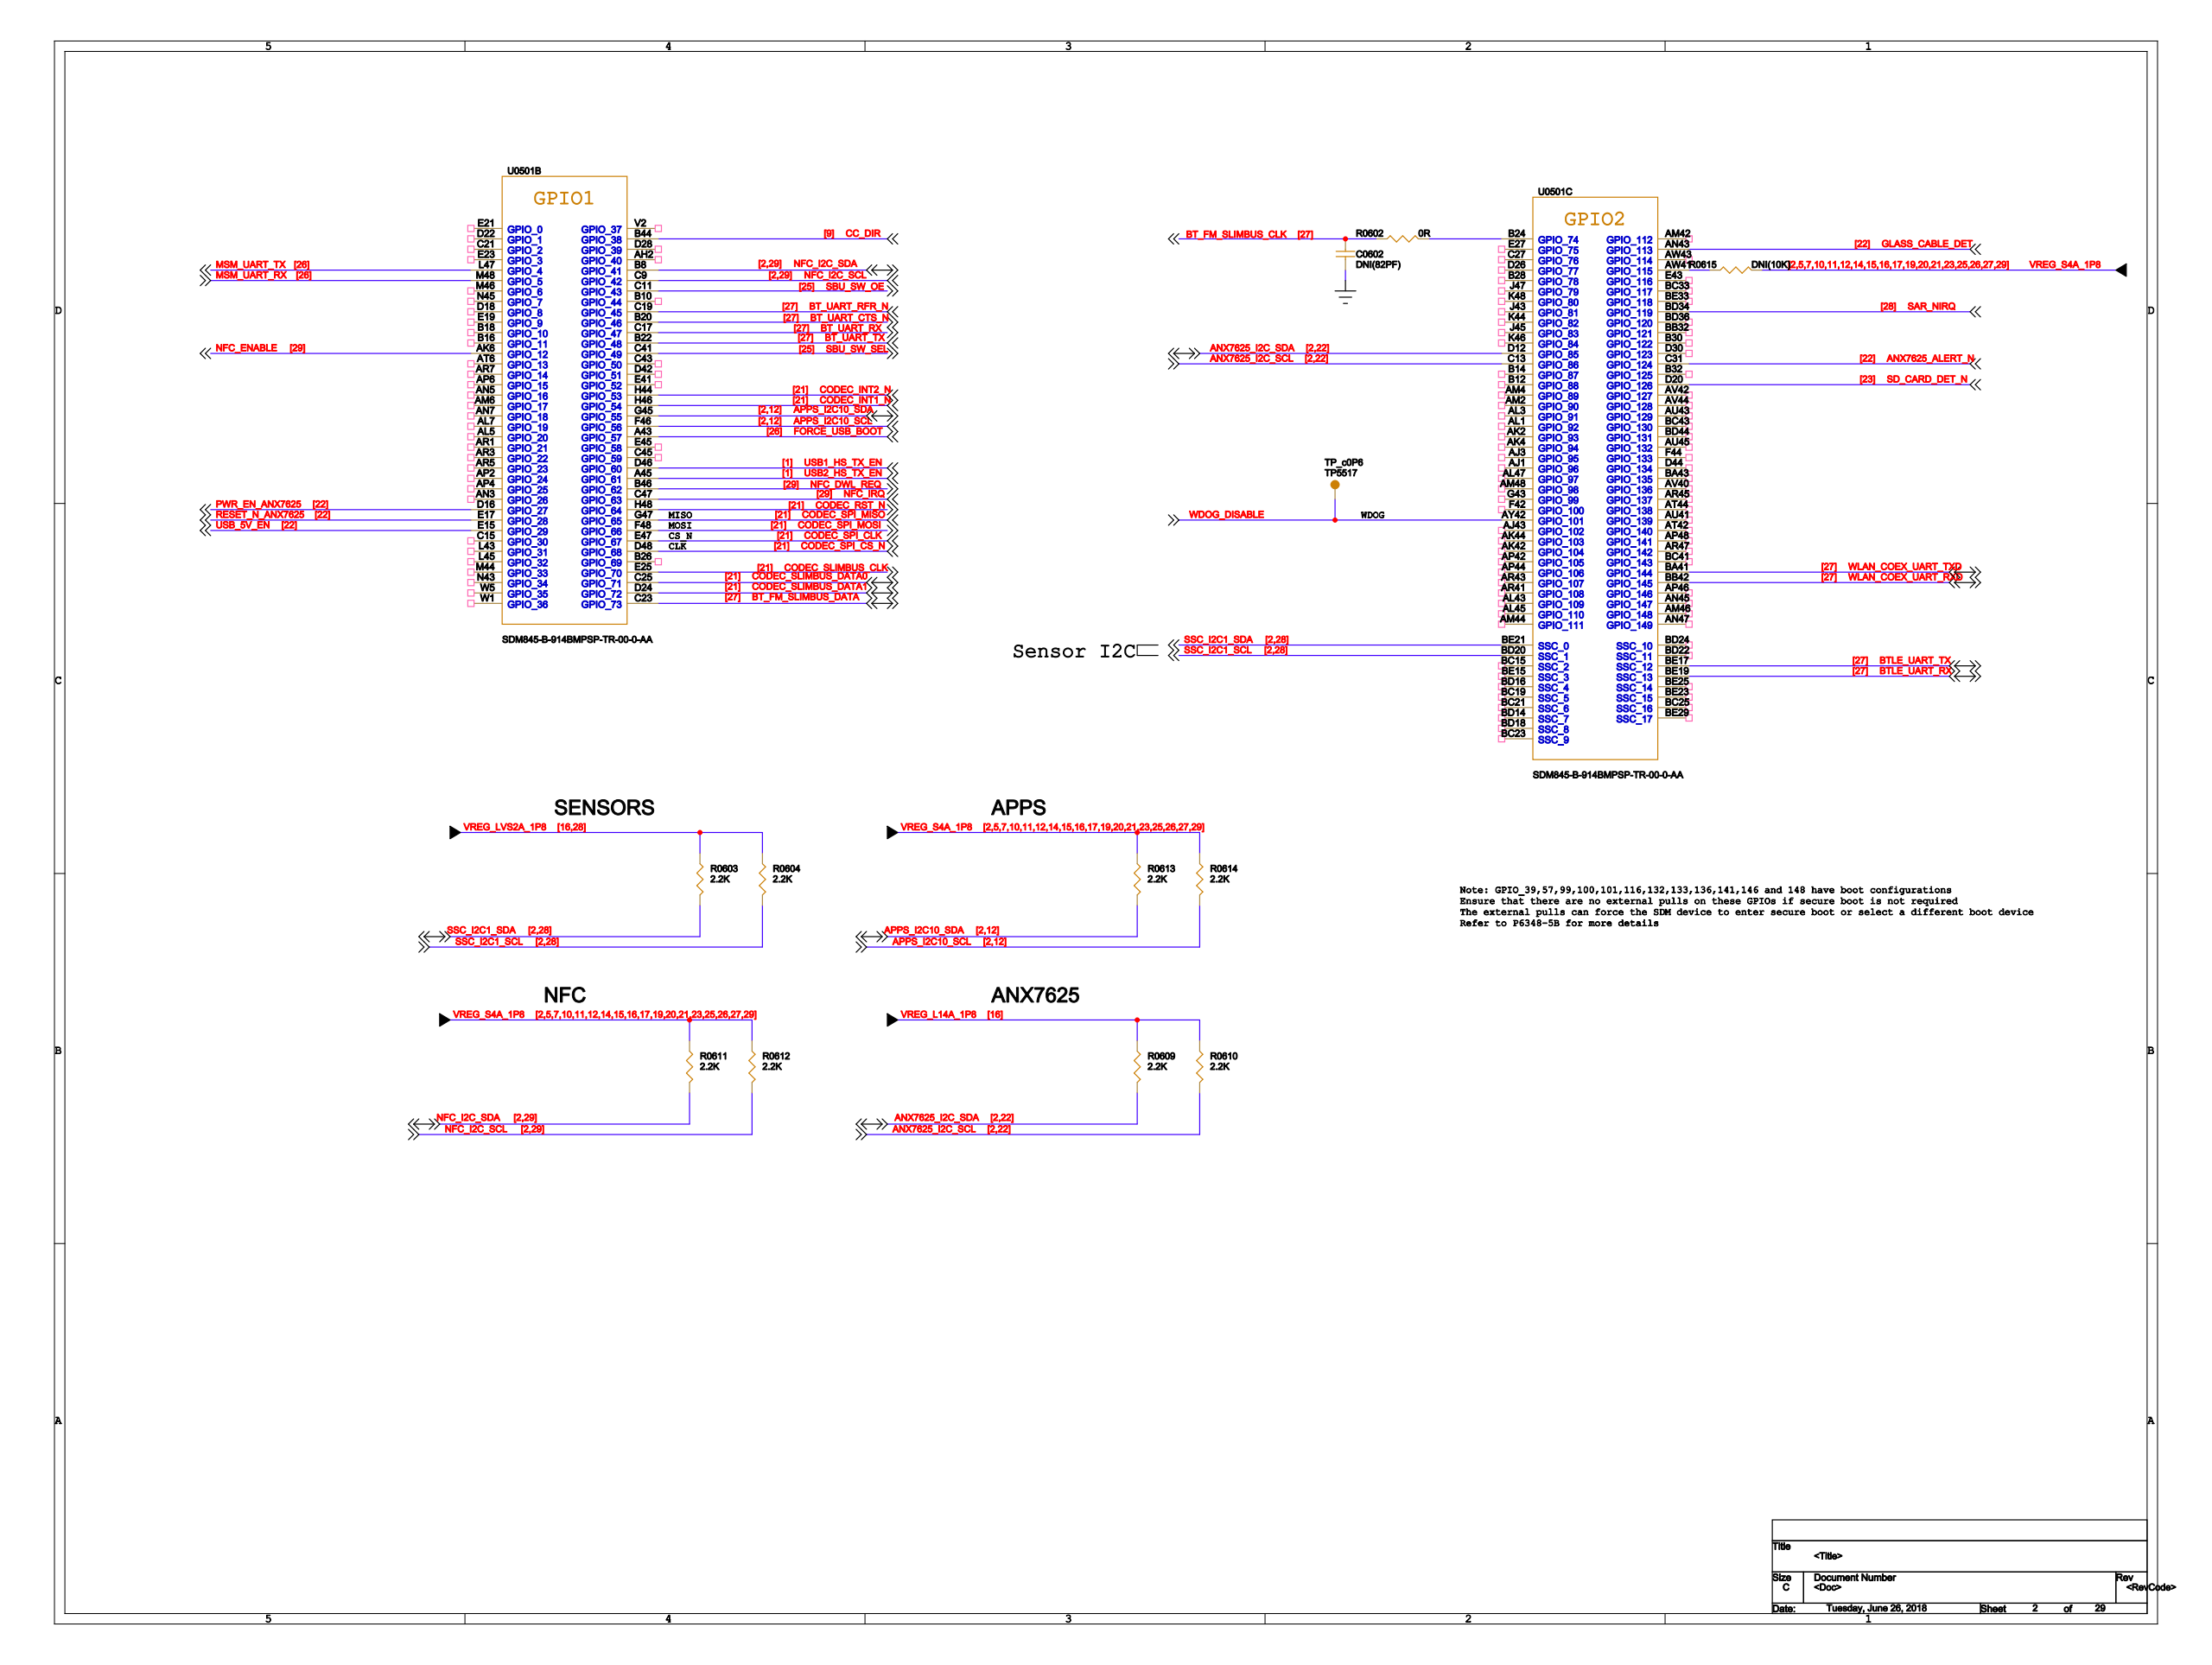Circuit board | Cadence Allegro | 802 parts | 566 nets | one sheet of the schematic
Parts on this sheet (reference | value | footprint):
C0602 | DNI(82PF) | C0402
R0602 | 0R | R0402
R0603 | 2.2K | R0201
R0604 | 2.2K | R0201
R0609 | 2.2K | R0201
R0610 | 2.2K | R0201
R0611 | 2.2K | R0201
R0612 | 2.2K | R0201
R0613 | 2.2K | R0201
R0614 | 2.2K | R0201
R0615 | DNI(10K) | R0201
TP5517 | TP_c0P6 | TP_C0P6
U0501 | SDM845-B-914BMPSP-TR-00-0-AA | BGA914_12P4X12P4_0P58_0P35
Nets of these parts (net: part-pin ...):
GND: C0602-2
VREG_S4A_1P8: R0611-1 R0612-1 R0613-1 R0614-1 R0615-2
VREG_LVS2A_1P8: R0603-1 R0604-1
SD_CARD_DET_N: U0501-D20
BT_FM_SLIMBUS_CLK: C0602-1 R0602-1
FORCE_USB_BOOT: U0501-A43
SSC_I2C1_SCL: R0604-2 U0501-BD20
SSC_I2C1_SDA: R0603-2 U0501-BE21
VREG_L14A_1P8: R0609-1 R0610-1
ANX7625_I2C_SDA: R0609-2 U0501-D12
ANX7625_I2C_SCL: R0610-2 U0501-C13
APPS_I2C10_SDA: R0613-2 U0501-G45
APPS_I2C10_SCL: R0614-2 U0501-F46
NFC_I2C_SDA: R0611-2 U0501-B8
NFC_I2C_SCL: R0612-2 U0501-C9
SBU_SW_OE: U0501-C11
SAR_NIRQ: U0501-BD34
N53596: R0615-1 U0501-AW41
USB_5V_EN: U0501-E15
NFC_ENABLE: U0501-AK6
ANX7625_ALERT_N: U0501-C31
WDOG_DISABLE: TP5517-1 U0501-AY42
CODEC_RST_N: U0501-H48
CODEC_SLIMBUS_DATA0: U0501-C25
CODEC_SLIMBUS_CLK: U0501-E25
CODEC_INT1_N: U0501-H46
CODEC_INT2_N: U0501-H44
NFC_IRQ: U0501-C47
NFC_DWL_REQ: U0501-B46
MSM_UART_TX: U0501-L47
MSM_UART_RX: U0501-M48
PWR_EN_ANX7625: U0501-D16
RESET_N_ANX7625: U0501-E17
CC_DIR: U0501-B44
BT_UART_RFR_N: U0501-C19
BT_UART_CTS_N: U0501-B20
BT_UART_RX: U0501-C17
BT_UART_TX: U0501-B22
SBU_SW_SEL: U0501-C41
USB1_HS_TX_EN: U0501-D46
USB2_HS_TX_EN: U0501-A45
CODEC_SPI_MISO: U0501-G47
CODEC_SPI_MOSI: U0501-F48
CODEC_SPI_CLK: U0501-E47
CODEC_SPI_CS_N: U0501-D48
CODEC_SLIMBUS_DATA1: U0501-D24
BT_FM_SLIMBUS_DATA: U0501-C23
GLASS_CABLE_DET: U0501-AN43
WLAN_COEX_UART_TXD: U0501-BA41
WLAN_COEX_UART_RXD: U0501-BB42
N52760: R0602-2 U0501-B24
BTLE_UART_TX: U0501-BE17
BTLE_UART_RX: U0501-BE19